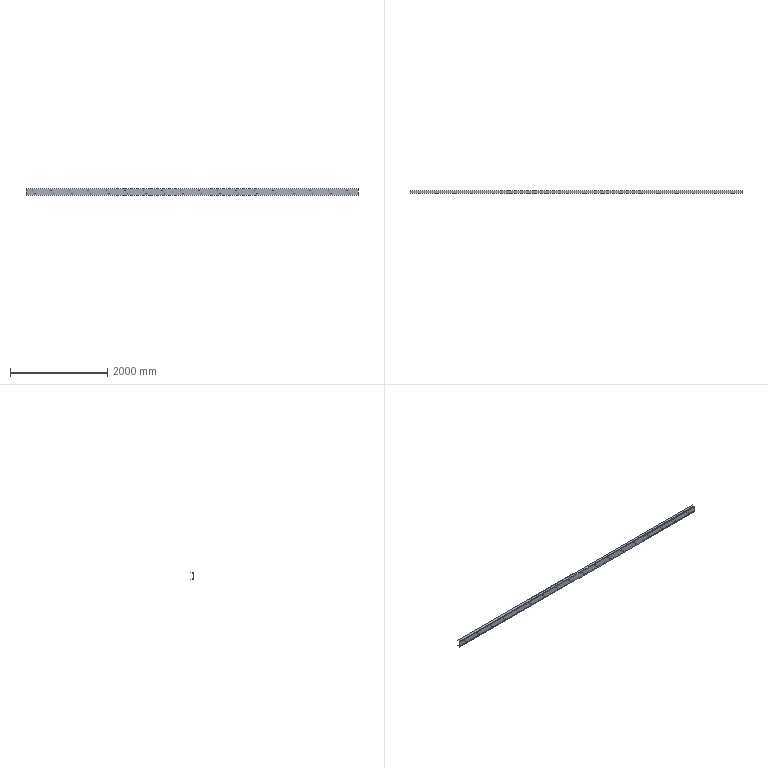Part | SolidWorks | features ICE 2, LPattern 1, WeldMemberFeat 1, WeldmentFeature 1 | 1 solid | 86 faces | box 6818 x 58 x 140 mm | volume 12457918 mm3 | cylinder 76 | plane 10 | commonest cylinder face diameters 16 x72 9.5 x2 19 x2